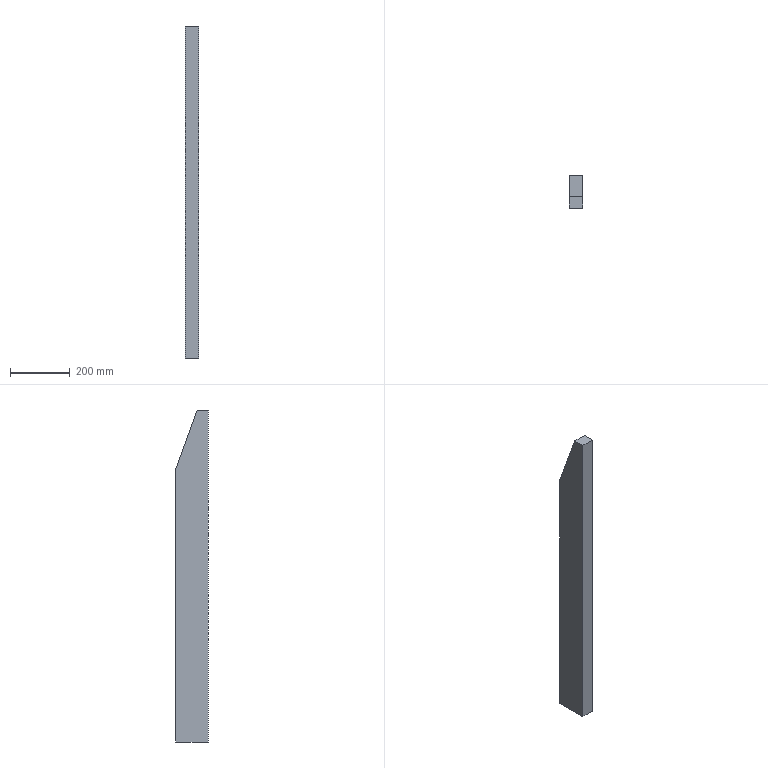Part | SolidWorks | features Extrusion 1 | 1 solid | 7 faces | box 45 x 110 x 1110 mm | volume 5170500 mm3 | plane 7
STEP:
#1=CARTESIAN_POINT('',(-22.5,38.,0.));
#2=VERTEX_POINT('',#1);
#3=CARTESIAN_POINT('',(-22.5,0.,0.));
#4=VERTEX_POINT('',#3);
#5=CARTESIAN_POINT('',(-22.5,38.,0.));
#6=DIRECTION('',(0.,-1.,0.));
#7=VECTOR('',#6,1000.);
#8=LINE('',#5,#7);
#9=EDGE_CURVE('',#2,#4,#8,.T.);
#10=ORIENTED_EDGE('',*,*,#9,.T.);
#11=CARTESIAN_POINT('',(22.5,0.,0.));
#12=VERTEX_POINT('',#11);
#13=CARTESIAN_POINT('',(22.5,0.,0.));
#14=DIRECTION('',(-1.,0.,0.));
#15=VECTOR('',#14,1000.);
#16=LINE('',#13,#15);
#17=EDGE_CURVE('',#12,#4,#16,.T.);
#18=ORIENTED_EDGE('',*,*,#17,.F.);
#19=CARTESIAN_POINT('',(22.5,38.,0.));
#20=VERTEX_POINT('',#19);
#21=CARTESIAN_POINT('',(22.5,38.,0.));
#22=DIRECTION('',(0.,-1.,0.));
#23=VECTOR('',#22,1000.);
#24=LINE('',#21,#23);
#25=EDGE_CURVE('',#20,#12,#24,.T.);
#26=ORIENTED_EDGE('',*,*,#25,.F.);
#27=CARTESIAN_POINT('',(22.5,38.,0.));
#28=DIRECTION('',(-1.,0.,0.));
#29=VECTOR('',#28,1000.);
#30=LINE('',#27,#29);
#31=EDGE_CURVE('',#20,#2,#30,.T.);
#32=ORIENTED_EDGE('',*,*,#31,.T.);
#33=EDGE_LOOP('',(#10,#18,#26,#32));
#34=FACE_OUTER_BOUND('',#33,.T.);
#35=CARTESIAN_POINT('',(22.5,38.,0.));
#36=DIRECTION('',(0.,0.,-1.));
#37=DIRECTION('',(0.,1.,0.));
#38=AXIS2_PLACEMENT_3D('',#35,#36,#37);
#39=PLANE('',#38);
#40=ADVANCED_FACE('',(#34),#39,.F.);
#41=CARTESIAN_POINT('',(-22.5,0.,-1110.));
#42=VERTEX_POINT('',#41);
#43=CARTESIAN_POINT('',(-22.5,0.,0.));
#44=DIRECTION('',(0.,0.,-1.));
#45=VECTOR('',#44,1000.);
#46=LINE('',#43,#45);
#47=EDGE_CURVE('',#4,#42,#46,.T.);
#48=ORIENTED_EDGE('',*,*,#47,.T.);
#49=CARTESIAN_POINT('',(22.5,0.,-1110.));
#50=VERTEX_POINT('',#49);
#51=CARTESIAN_POINT('',(22.5,0.,-1110.));
#52=DIRECTION('',(-1.,0.,0.));
#53=VECTOR('',#52,1000.);
#54=LINE('',#51,#53);
#55=EDGE_CURVE('',#50,#42,#54,.T.);
#56=ORIENTED_EDGE('',*,*,#55,.F.);
#57=CARTESIAN_POINT('',(22.5,0.,0.));
#58=DIRECTION('',(0.,0.,-1.));
#59=VECTOR('',#58,1000.);
#60=LINE('',#57,#59);
#61=EDGE_CURVE('',#12,#50,#60,.T.);
#62=ORIENTED_EDGE('',*,*,#61,.F.);
#63=ORIENTED_EDGE('',*,*,#17,.T.);
#64=EDGE_LOOP('',(#48,#56,#62,#63));
#65=FACE_OUTER_BOUND('',#64,.T.);
#66=CARTESIAN_POINT('',(22.5,0.,0.));
#67=DIRECTION('',(0.,1.,0.));
#68=DIRECTION('',(0.,0.,1.));
#69=AXIS2_PLACEMENT_3D('',#66,#67,#68);
#70=PLANE('',#69);
#71=ADVANCED_FACE('',(#65),#70,.F.);
#72=CARTESIAN_POINT('',(-22.5,110.,-1110.));
#73=VERTEX_POINT('',#72);
#74=CARTESIAN_POINT('',(-22.5,0.,-1110.));
#75=DIRECTION('',(0.,1.,0.));
#76=VECTOR('',#75,1000.);
#77=LINE('',#74,#76);
#78=EDGE_CURVE('',#42,#73,#77,.T.);
#79=ORIENTED_EDGE('',*,*,#78,.T.);
#80=CARTESIAN_POINT('',(22.5,110.,-1110.));
#81=VERTEX_POINT('',#80);
#82=CARTESIAN_POINT('',(22.5,110.,-1110.));
#83=DIRECTION('',(-1.,0.,0.));
#84=VECTOR('',#83,1000.);
#85=LINE('',#82,#84);
#86=EDGE_CURVE('',#81,#73,#85,.T.);
#87=ORIENTED_EDGE('',*,*,#86,.F.);
#88=CARTESIAN_POINT('',(22.5,0.,-1110.));
#89=DIRECTION('',(0.,1.,0.));
#90=VECTOR('',#89,1000.);
#91=LINE('',#88,#90);
#92=EDGE_CURVE('',#50,#81,#91,.T.);
#93=ORIENTED_EDGE('',*,*,#92,.F.);
#94=ORIENTED_EDGE('',*,*,#55,.T.);
#95=EDGE_LOOP('',(#79,#87,#93,#94));
#96=FACE_OUTER_BOUND('',#95,.T.);
#97=CARTESIAN_POINT('',(22.5,0.,-1110.));
#98=DIRECTION('',(0.,0.,1.));
#99=DIRECTION('',(1.,0.,0.));
#100=AXIS2_PLACEMENT_3D('',#97,#98,#99);
#101=PLANE('',#100);
#102=ADVANCED_FACE('',(#96),#101,.F.);
#103=CARTESIAN_POINT('',(-22.5,110.,-200.));
#104=VERTEX_POINT('',#103);
#105=CARTESIAN_POINT('',(-22.5,110.,-1110.));
#106=DIRECTION('',(0.,0.,1.));
#107=VECTOR('',#106,1000.);
#108=LINE('',#105,#107);
#109=EDGE_CURVE('',#73,#104,#108,.T.);
#110=ORIENTED_EDGE('',*,*,#109,.T.);
#111=CARTESIAN_POINT('',(22.5,110.,-200.));
#112=VERTEX_POINT('',#111);
#113=CARTESIAN_POINT('',(22.5,110.,-200.));
#114=DIRECTION('',(-1.,0.,0.));
#115=VECTOR('',#114,1000.);
#116=LINE('',#113,#115);
#117=EDGE_CURVE('',#112,#104,#116,.T.);
#118=ORIENTED_EDGE('',*,*,#117,.F.);
#119=CARTESIAN_POINT('',(22.5,110.,-1110.));
#120=DIRECTION('',(0.,0.,1.));
#121=VECTOR('',#120,1000.);
#122=LINE('',#119,#121);
#123=EDGE_CURVE('',#81,#112,#122,.T.);
#124=ORIENTED_EDGE('',*,*,#123,.F.);
#125=ORIENTED_EDGE('',*,*,#86,.T.);
#126=EDGE_LOOP('',(#110,#118,#124,#125));
#127=FACE_OUTER_BOUND('',#126,.T.);
#128=CARTESIAN_POINT('',(22.5,110.,-1110.));
#129=DIRECTION('',(0.,-1.,0.));
#130=DIRECTION('',(0.,0.,-1.));
#131=AXIS2_PLACEMENT_3D('',#128,#129,#130);
#132=PLANE('',#131);
#133=ADVANCED_FACE('',(#127),#132,.F.);
#134=CARTESIAN_POINT('',(-22.5,110.,-200.));
#135=DIRECTION('',(0.,-0.3387,0.9409));
#136=VECTOR('',#135,1000.);
#137=LINE('',#134,#136);
#138=EDGE_CURVE('',#104,#2,#137,.T.);
#139=ORIENTED_EDGE('',*,*,#138,.T.);
#140=ORIENTED_EDGE('',*,*,#31,.F.);
#141=CARTESIAN_POINT('',(22.5,110.,-200.));
#142=DIRECTION('',(0.,-0.3387,0.9409));
#143=VECTOR('',#142,1000.);
#144=LINE('',#141,#143);
#145=EDGE_CURVE('',#112,#20,#144,.T.);
#146=ORIENTED_EDGE('',*,*,#145,.F.);
#147=ORIENTED_EDGE('',*,*,#117,.T.);
#148=EDGE_LOOP('',(#139,#140,#146,#147));
#149=FACE_OUTER_BOUND('',#148,.T.);
#150=CARTESIAN_POINT('',(22.5,110.,-200.));
#151=DIRECTION('',(0.,-0.9409,-0.3387));
#152=DIRECTION('',(0.,0.3387,-0.9409));
#153=AXIS2_PLACEMENT_3D('',#150,#151,#152);
#154=PLANE('',#153);
#155=ADVANCED_FACE('',(#149),#154,.F.);
#156=ORIENTED_EDGE('',*,*,#25,.T.);
#157=ORIENTED_EDGE('',*,*,#61,.T.);
#158=ORIENTED_EDGE('',*,*,#92,.T.);
#159=ORIENTED_EDGE('',*,*,#123,.T.);
#160=ORIENTED_EDGE('',*,*,#145,.T.);
#161=EDGE_LOOP('',(#156,#157,#158,#159,#160));
#162=FACE_OUTER_BOUND('',#161,.T.);
#163=CARTESIAN_POINT('',(22.5,0.,0.));
#164=DIRECTION('',(1.,0.,0.));
#165=DIRECTION('',(0.,0.,-1.));
#166=AXIS2_PLACEMENT_3D('',#163,#164,#165);
#167=PLANE('',#166);
#168=ADVANCED_FACE('',(#162),#167,.T.);
#169=ORIENTED_EDGE('',*,*,#9,.F.);
#170=ORIENTED_EDGE('',*,*,#138,.F.);
#171=ORIENTED_EDGE('',*,*,#109,.F.);
#172=ORIENTED_EDGE('',*,*,#78,.F.);
#173=ORIENTED_EDGE('',*,*,#47,.F.);
#174=EDGE_LOOP('',(#169,#170,#171,#172,#173));
#175=FACE_OUTER_BOUND('',#174,.T.);
#176=CARTESIAN_POINT('',(-22.5,0.,0.));
#177=DIRECTION('',(1.,0.,0.));
#178=DIRECTION('',(0.,0.,-1.));
#179=AXIS2_PLACEMENT_3D('',#176,#177,#178);
#180=PLANE('',#179);
#181=ADVANCED_FACE('',(#175),#180,.F.);
#182=CLOSED_SHELL('',(#40,#71,#102,#133,#155,#168,#181));
#183=MANIFOLD_SOLID_BREP('',#182);
#184=CARTESIAN_POINT('',(0.,0.,0.));
#185=DIRECTION('',(0.,0.,1.));
#186=DIRECTION('',(1.,0.,0.));
#187=AXIS2_PLACEMENT_3D('',#184,#185,#186);
#188=(LENGTH_UNIT()NAMED_UNIT(*)SI_UNIT(.MILLI.,.METRE.));
#189=UNCERTAINTY_MEASURE_WITH_UNIT(LENGTH_MEASURE(0.00001),#188,'','');
#190=(NAMED_UNIT(*)PLANE_ANGLE_UNIT()SI_UNIT($,.RADIAN.));
#191=(NAMED_UNIT(*)SI_UNIT($,.STERADIAN.)SOLID_ANGLE_UNIT());
#192=(GEOMETRIC_REPRESENTATION_CONTEXT(3)GLOBAL_UNCERTAINTY_ASSIGNED_CONTEXT((#189))GLOBAL_UNIT_ASSIGNED_CONTEXT((#188,#190,#191))REPRESENTATION_CONTEXT('',''));
#193=ADVANCED_BREP_SHAPE_REPRESENTATION('',(#183,#187),#192);